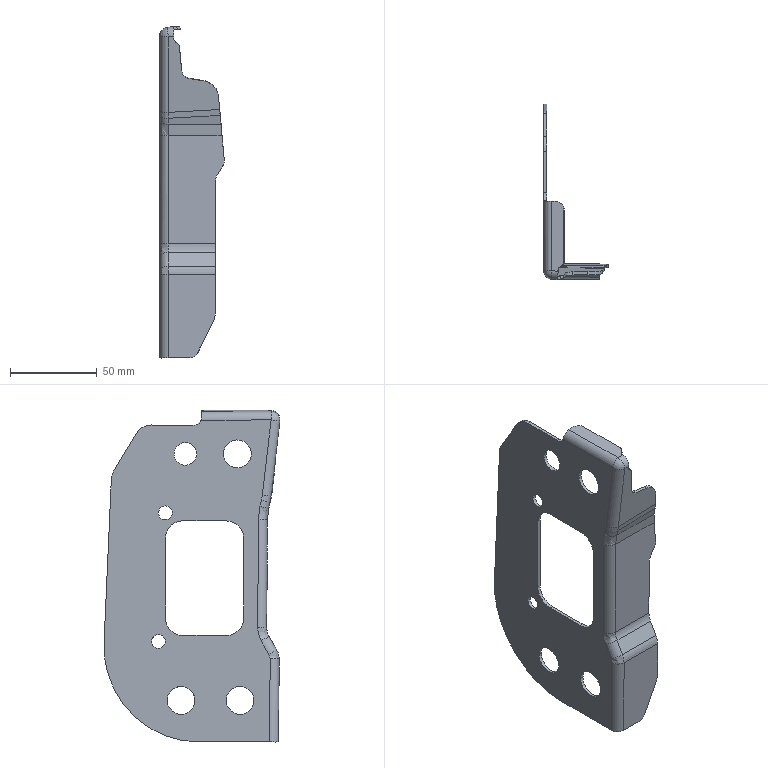Part | 1 solid | 108 faces | box 37.255 x 101.381 x 191.221 mm | volume 32940 mm3 | spline 52 | cylinder 27 | other 15 | plane 12 | sphere 2 | commonest cylinder face diameters 10 x8 6.4 x7 20 x4 60 x2 6 x1 16.4 x1